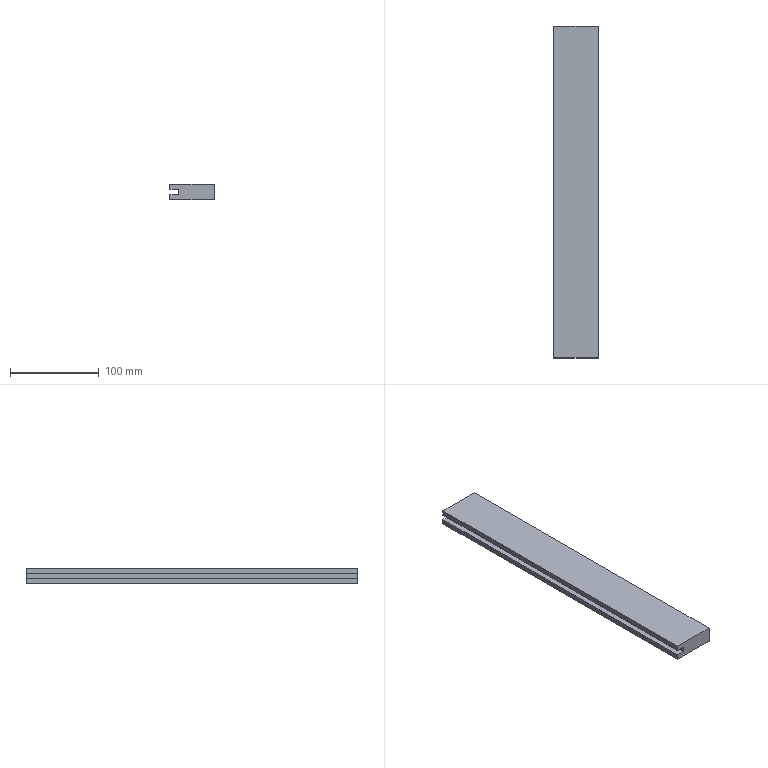Part | STEP file | Superstructure_1 | 1 solid | 10 faces | box 50 x 374 x 18 mm | volume 314160 mm3 | plane 10
STEP:
#1=CARTESIAN_POINT('',(0.,0.,0.));
#2=DIRECTION('',(0.,0.,1.));
#3=DIRECTION('',(1.,0.,0.));
#4=AXIS2_PLACEMENT_3D('',#1,#2,#3);
#5=CARTESIAN_POINT('',(-25.,187.,-3.));
#6=VERTEX_POINT('',#5);
#7=CARTESIAN_POINT('',(-25.,-187.,-3.));
#8=VERTEX_POINT('',#7);
#9=CARTESIAN_POINT('',(-25.,187.,-3.));
#10=DIRECTION('',(0.,-1.,0.));
#11=VECTOR('',#10,1.);
#12=LINE('',#9,#11);
#13=CARTESIAN_POINT('',(-25.,187.,-3.));
#14=DIRECTION('',(1.,0.,0.));
#15=DIRECTION('',(0.,0.,-1.));
#16=AXIS2_PLACEMENT_3D('',#13,#14,#15);
#17=PLANE('',#16);
#18=CARTESIAN_POINT('',(0.,0.));
#19=DIRECTION('',(0.,-1.));
#20=VECTOR('',#19,1.);
#21=LINE('',#18,#20);
#22=(GEOMETRIC_REPRESENTATION_CONTEXT(2)PARAMETRIC_REPRESENTATION_CONTEXT()REPRESENTATION_CONTEXT('',''));
#23=DEFINITIONAL_REPRESENTATION('',(#21),#22);
#24=PCURVE('',#17,#23);
#25=CARTESIAN_POINT('',(-25.,187.,-3.));
#26=DIRECTION('',(0.,0.,1.));
#27=DIRECTION('',(1.,0.,0.));
#28=AXIS2_PLACEMENT_3D('',#25,#26,#27);
#29=PLANE('',#28);
#30=CARTESIAN_POINT('',(0.,0.));
#31=DIRECTION('',(0.,-1.));
#32=VECTOR('',#31,1.);
#33=LINE('',#30,#32);
#34=(GEOMETRIC_REPRESENTATION_CONTEXT(2)PARAMETRIC_REPRESENTATION_CONTEXT()REPRESENTATION_CONTEXT('',''));
#35=DEFINITIONAL_REPRESENTATION('',(#33),#34);
#36=PCURVE('',#29,#35);
#37=SURFACE_CURVE('',#12,(#24,#36),.PCURVE_S1.);
#38=EDGE_CURVE('',#6,#8,#37,.T.);
#39=ORIENTED_EDGE('',*,*,#38,.T.);
#40=CARTESIAN_POINT('',(-25.,-187.,-9.));
#41=VERTEX_POINT('',#40);
#42=CARTESIAN_POINT('',(-25.,-187.,-3.));
#43=DIRECTION('',(0.,0.,-1.));
#44=VECTOR('',#43,1.);
#45=LINE('',#42,#44);
#46=CARTESIAN_POINT('',(0.,-374.));
#47=DIRECTION('',(1.,0.));
#48=VECTOR('',#47,1.);
#49=LINE('',#46,#48);
#50=(GEOMETRIC_REPRESENTATION_CONTEXT(2)PARAMETRIC_REPRESENTATION_CONTEXT()REPRESENTATION_CONTEXT('',''));
#51=DEFINITIONAL_REPRESENTATION('',(#49),#50);
#52=PCURVE('',#17,#51);
#53=CARTESIAN_POINT('',(-2.179,-187.,0.));
#54=DIRECTION('',(0.,1.,0.));
#55=DIRECTION('',(0.,0.,1.));
#56=AXIS2_PLACEMENT_3D('',#53,#54,#55);
#57=PLANE('',#56);
#58=CARTESIAN_POINT('',(-3.,-22.821));
#59=DIRECTION('',(-1.,0.));
#60=VECTOR('',#59,1.);
#61=LINE('',#58,#60);
#62=(GEOMETRIC_REPRESENTATION_CONTEXT(2)PARAMETRIC_REPRESENTATION_CONTEXT()REPRESENTATION_CONTEXT('',''));
#63=DEFINITIONAL_REPRESENTATION('',(#61),#62);
#64=PCURVE('',#57,#63);
#65=SURFACE_CURVE('',#45,(#52,#64),.PCURVE_S1.);
#66=EDGE_CURVE('',#8,#41,#65,.T.);
#67=ORIENTED_EDGE('',*,*,#66,.T.);
#68=CARTESIAN_POINT('',(-25.,187.,-9.));
#69=VERTEX_POINT('',#68);
#70=CARTESIAN_POINT('',(-25.,187.,-9.));
#71=DIRECTION('',(0.,-1.,0.));
#72=VECTOR('',#71,1.);
#73=LINE('',#70,#72);
#74=CARTESIAN_POINT('',(6.,0.));
#75=DIRECTION('',(0.,-1.));
#76=VECTOR('',#75,1.);
#77=LINE('',#74,#76);
#78=(GEOMETRIC_REPRESENTATION_CONTEXT(2)PARAMETRIC_REPRESENTATION_CONTEXT()REPRESENTATION_CONTEXT('',''));
#79=DEFINITIONAL_REPRESENTATION('',(#77),#78);
#80=PCURVE('',#17,#79);
#81=CARTESIAN_POINT('',(-25.,187.,-9.));
#82=DIRECTION('',(0.,0.,1.));
#83=DIRECTION('',(1.,0.,0.));
#84=AXIS2_PLACEMENT_3D('',#81,#82,#83);
#85=PLANE('',#84);
#86=CARTESIAN_POINT('',(0.,0.));
#87=DIRECTION('',(0.,-1.));
#88=VECTOR('',#87,1.);
#89=LINE('',#86,#88);
#90=(GEOMETRIC_REPRESENTATION_CONTEXT(2)PARAMETRIC_REPRESENTATION_CONTEXT()REPRESENTATION_CONTEXT('',''));
#91=DEFINITIONAL_REPRESENTATION('',(#89),#90);
#92=PCURVE('',#85,#91);
#93=SURFACE_CURVE('',#73,(#80,#92),.PCURVE_S1.);
#94=EDGE_CURVE('',#69,#41,#93,.T.);
#95=ORIENTED_EDGE('',*,*,#94,.F.);
#96=CARTESIAN_POINT('',(-25.,187.,-3.));
#97=DIRECTION('',(0.,0.,-1.));
#98=VECTOR('',#97,1.);
#99=LINE('',#96,#98);
#100=CARTESIAN_POINT('',(0.,0.));
#101=DIRECTION('',(1.,0.));
#102=VECTOR('',#101,1.);
#103=LINE('',#100,#102);
#104=(GEOMETRIC_REPRESENTATION_CONTEXT(2)PARAMETRIC_REPRESENTATION_CONTEXT()REPRESENTATION_CONTEXT('',''));
#105=DEFINITIONAL_REPRESENTATION('',(#103),#104);
#106=PCURVE('',#17,#105);
#107=CARTESIAN_POINT('',(-2.179,187.,0.));
#108=DIRECTION('',(0.,1.,0.));
#109=DIRECTION('',(0.,0.,1.));
#110=AXIS2_PLACEMENT_3D('',#107,#108,#109);
#111=PLANE('',#110);
#112=CARTESIAN_POINT('',(-3.,-22.821));
#113=DIRECTION('',(-1.,0.));
#114=VECTOR('',#113,1.);
#115=LINE('',#112,#114);
#116=(GEOMETRIC_REPRESENTATION_CONTEXT(2)PARAMETRIC_REPRESENTATION_CONTEXT()REPRESENTATION_CONTEXT('',''));
#117=DEFINITIONAL_REPRESENTATION('',(#115),#116);
#118=PCURVE('',#111,#117);
#119=SURFACE_CURVE('',#99,(#106,#118),.PCURVE_S1.);
#120=EDGE_CURVE('',#6,#69,#119,.T.);
#121=ORIENTED_EDGE('',*,*,#120,.F.);
#122=EDGE_LOOP('',(#39,#67,#95,#121));
#123=FACE_BOUND('',#122,.F.);
#124=ADVANCED_FACE('',(#123),#17,.F.);
#125=ORIENTED_EDGE('',*,*,#94,.T.);
#126=CARTESIAN_POINT('',(25.,-187.,-9.));
#127=VERTEX_POINT('',#126);
#128=CARTESIAN_POINT('',(-25.,-187.,-9.));
#129=DIRECTION('',(1.,0.,0.));
#130=VECTOR('',#129,1.);
#131=LINE('',#128,#130);
#132=CARTESIAN_POINT('',(0.,-374.));
#133=DIRECTION('',(1.,0.));
#134=VECTOR('',#133,1.);
#135=LINE('',#132,#134);
#136=(GEOMETRIC_REPRESENTATION_CONTEXT(2)PARAMETRIC_REPRESENTATION_CONTEXT()REPRESENTATION_CONTEXT('',''));
#137=DEFINITIONAL_REPRESENTATION('',(#135),#136);
#138=PCURVE('',#85,#137);
#139=CARTESIAN_POINT('',(-9.,-22.821));
#140=DIRECTION('',(0.,1.));
#141=VECTOR('',#140,1.);
#142=LINE('',#139,#141);
#143=(GEOMETRIC_REPRESENTATION_CONTEXT(2)PARAMETRIC_REPRESENTATION_CONTEXT()REPRESENTATION_CONTEXT('',''));
#144=DEFINITIONAL_REPRESENTATION('',(#142),#143);
#145=PCURVE('',#57,#144);
#146=SURFACE_CURVE('',#131,(#138,#145),.PCURVE_S1.);
#147=EDGE_CURVE('',#41,#127,#146,.T.);
#148=ORIENTED_EDGE('',*,*,#147,.T.);
#149=CARTESIAN_POINT('',(25.,187.,-9.));
#150=VERTEX_POINT('',#149);
#151=CARTESIAN_POINT('',(25.,187.,-9.));
#152=DIRECTION('',(0.,-1.,0.));
#153=VECTOR('',#152,1.);
#154=LINE('',#151,#153);
#155=CARTESIAN_POINT('',(50.,0.));
#156=DIRECTION('',(0.,-1.));
#157=VECTOR('',#156,1.);
#158=LINE('',#155,#157);
#159=(GEOMETRIC_REPRESENTATION_CONTEXT(2)PARAMETRIC_REPRESENTATION_CONTEXT()REPRESENTATION_CONTEXT('',''));
#160=DEFINITIONAL_REPRESENTATION('',(#158),#159);
#161=PCURVE('',#85,#160);
#162=CARTESIAN_POINT('',(25.,187.,-9.));
#163=DIRECTION('',(-1.,0.,0.));
#164=DIRECTION('',(0.,0.,1.));
#165=AXIS2_PLACEMENT_3D('',#162,#163,#164);
#166=PLANE('',#165);
#167=CARTESIAN_POINT('',(0.,0.));
#168=DIRECTION('',(0.,-1.));
#169=VECTOR('',#168,1.);
#170=LINE('',#167,#169);
#171=(GEOMETRIC_REPRESENTATION_CONTEXT(2)PARAMETRIC_REPRESENTATION_CONTEXT()REPRESENTATION_CONTEXT('',''));
#172=DEFINITIONAL_REPRESENTATION('',(#170),#171);
#173=PCURVE('',#166,#172);
#174=SURFACE_CURVE('',#154,(#161,#173),.PCURVE_S1.);
#175=EDGE_CURVE('',#150,#127,#174,.T.);
#176=ORIENTED_EDGE('',*,*,#175,.F.);
#177=CARTESIAN_POINT('',(-25.,187.,-9.));
#178=DIRECTION('',(1.,0.,0.));
#179=VECTOR('',#178,1.);
#180=LINE('',#177,#179);
#181=CARTESIAN_POINT('',(0.,0.));
#182=DIRECTION('',(1.,0.));
#183=VECTOR('',#182,1.);
#184=LINE('',#181,#183);
#185=(GEOMETRIC_REPRESENTATION_CONTEXT(2)PARAMETRIC_REPRESENTATION_CONTEXT()REPRESENTATION_CONTEXT('',''));
#186=DEFINITIONAL_REPRESENTATION('',(#184),#185);
#187=PCURVE('',#85,#186);
#188=CARTESIAN_POINT('',(-9.,-22.821));
#189=DIRECTION('',(0.,1.));
#190=VECTOR('',#189,1.);
#191=LINE('',#188,#190);
#192=(GEOMETRIC_REPRESENTATION_CONTEXT(2)PARAMETRIC_REPRESENTATION_CONTEXT()REPRESENTATION_CONTEXT('',''));
#193=DEFINITIONAL_REPRESENTATION('',(#191),#192);
#194=PCURVE('',#111,#193);
#195=SURFACE_CURVE('',#180,(#187,#194),.PCURVE_S1.);
#196=EDGE_CURVE('',#69,#150,#195,.T.);
#197=ORIENTED_EDGE('',*,*,#196,.F.);
#198=EDGE_LOOP('',(#125,#148,#176,#197));
#199=FACE_BOUND('',#198,.F.);
#200=ADVANCED_FACE('',(#199),#85,.F.);
#201=ORIENTED_EDGE('',*,*,#175,.T.);
#202=CARTESIAN_POINT('',(25.,-187.,9.));
#203=VERTEX_POINT('',#202);
#204=CARTESIAN_POINT('',(25.,-187.,-9.));
#205=DIRECTION('',(0.,0.,1.));
#206=VECTOR('',#205,1.);
#207=LINE('',#204,#206);
#208=CARTESIAN_POINT('',(0.,-374.));
#209=DIRECTION('',(1.,0.));
#210=VECTOR('',#209,1.);
#211=LINE('',#208,#210);
#212=(GEOMETRIC_REPRESENTATION_CONTEXT(2)PARAMETRIC_REPRESENTATION_CONTEXT()REPRESENTATION_CONTEXT('',''));
#213=DEFINITIONAL_REPRESENTATION('',(#211),#212);
#214=PCURVE('',#166,#213);
#215=CARTESIAN_POINT('',(-9.,27.179));
#216=DIRECTION('',(1.,0.));
#217=VECTOR('',#216,1.);
#218=LINE('',#215,#217);
#219=(GEOMETRIC_REPRESENTATION_CONTEXT(2)PARAMETRIC_REPRESENTATION_CONTEXT()REPRESENTATION_CONTEXT('',''));
#220=DEFINITIONAL_REPRESENTATION('',(#218),#219);
#221=PCURVE('',#57,#220);
#222=SURFACE_CURVE('',#207,(#214,#221),.PCURVE_S1.);
#223=EDGE_CURVE('',#127,#203,#222,.T.);
#224=ORIENTED_EDGE('',*,*,#223,.T.);
#225=CARTESIAN_POINT('',(25.,187.,9.));
#226=VERTEX_POINT('',#225);
#227=CARTESIAN_POINT('',(25.,187.,9.));
#228=DIRECTION('',(0.,-1.,0.));
#229=VECTOR('',#228,1.);
#230=LINE('',#227,#229);
#231=CARTESIAN_POINT('',(18.,0.));
#232=DIRECTION('',(0.,-1.));
#233=VECTOR('',#232,1.);
#234=LINE('',#231,#233);
#235=(GEOMETRIC_REPRESENTATION_CONTEXT(2)PARAMETRIC_REPRESENTATION_CONTEXT()REPRESENTATION_CONTEXT('',''));
#236=DEFINITIONAL_REPRESENTATION('',(#234),#235);
#237=PCURVE('',#166,#236);
#238=CARTESIAN_POINT('',(25.,187.,9.));
#239=DIRECTION('',(0.,0.,-1.));
#240=DIRECTION('',(-1.,0.,0.));
#241=AXIS2_PLACEMENT_3D('',#238,#239,#240);
#242=PLANE('',#241);
#243=CARTESIAN_POINT('',(0.,0.));
#244=DIRECTION('',(0.,-1.));
#245=VECTOR('',#244,1.);
#246=LINE('',#243,#245);
#247=(GEOMETRIC_REPRESENTATION_CONTEXT(2)PARAMETRIC_REPRESENTATION_CONTEXT()REPRESENTATION_CONTEXT('',''));
#248=DEFINITIONAL_REPRESENTATION('',(#246),#247);
#249=PCURVE('',#242,#248);
#250=SURFACE_CURVE('',#230,(#237,#249),.PCURVE_S1.);
#251=EDGE_CURVE('',#226,#203,#250,.T.);
#252=ORIENTED_EDGE('',*,*,#251,.F.);
#253=CARTESIAN_POINT('',(25.,187.,-9.));
#254=DIRECTION('',(0.,0.,1.));
#255=VECTOR('',#254,1.);
#256=LINE('',#253,#255);
#257=CARTESIAN_POINT('',(0.,0.));
#258=DIRECTION('',(1.,0.));
#259=VECTOR('',#258,1.);
#260=LINE('',#257,#259);
#261=(GEOMETRIC_REPRESENTATION_CONTEXT(2)PARAMETRIC_REPRESENTATION_CONTEXT()REPRESENTATION_CONTEXT('',''));
#262=DEFINITIONAL_REPRESENTATION('',(#260),#261);
#263=PCURVE('',#166,#262);
#264=CARTESIAN_POINT('',(-9.,27.179));
#265=DIRECTION('',(1.,0.));
#266=VECTOR('',#265,1.);
#267=LINE('',#264,#266);
#268=(GEOMETRIC_REPRESENTATION_CONTEXT(2)PARAMETRIC_REPRESENTATION_CONTEXT()REPRESENTATION_CONTEXT('',''));
#269=DEFINITIONAL_REPRESENTATION('',(#267),#268);
#270=PCURVE('',#111,#269);
#271=SURFACE_CURVE('',#256,(#263,#270),.PCURVE_S1.);
#272=EDGE_CURVE('',#150,#226,#271,.T.);
#273=ORIENTED_EDGE('',*,*,#272,.F.);
#274=EDGE_LOOP('',(#201,#224,#252,#273));
#275=FACE_BOUND('',#274,.F.);
#276=ADVANCED_FACE('',(#275),#166,.F.);
#277=ORIENTED_EDGE('',*,*,#251,.T.);
#278=CARTESIAN_POINT('',(-25.,-187.,9.));
#279=VERTEX_POINT('',#278);
#280=CARTESIAN_POINT('',(25.,-187.,9.));
#281=DIRECTION('',(-1.,0.,0.));
#282=VECTOR('',#281,1.);
#283=LINE('',#280,#282);
#284=CARTESIAN_POINT('',(0.,-374.));
#285=DIRECTION('',(1.,0.));
#286=VECTOR('',#285,1.);
#287=LINE('',#284,#286);
#288=(GEOMETRIC_REPRESENTATION_CONTEXT(2)PARAMETRIC_REPRESENTATION_CONTEXT()REPRESENTATION_CONTEXT('',''));
#289=DEFINITIONAL_REPRESENTATION('',(#287),#288);
#290=PCURVE('',#242,#289);
#291=CARTESIAN_POINT('',(9.,27.179));
#292=DIRECTION('',(0.,-1.));
#293=VECTOR('',#292,1.);
#294=LINE('',#291,#293);
#295=(GEOMETRIC_REPRESENTATION_CONTEXT(2)PARAMETRIC_REPRESENTATION_CONTEXT()REPRESENTATION_CONTEXT('',''));
#296=DEFINITIONAL_REPRESENTATION('',(#294),#295);
#297=PCURVE('',#57,#296);
#298=SURFACE_CURVE('',#283,(#290,#297),.PCURVE_S1.);
#299=EDGE_CURVE('',#203,#279,#298,.T.);
#300=ORIENTED_EDGE('',*,*,#299,.T.);
#301=CARTESIAN_POINT('',(-25.,187.,9.));
#302=VERTEX_POINT('',#301);
#303=CARTESIAN_POINT('',(-25.,187.,9.));
#304=DIRECTION('',(0.,-1.,0.));
#305=VECTOR('',#304,1.);
#306=LINE('',#303,#305);
#307=CARTESIAN_POINT('',(50.,0.));
#308=DIRECTION('',(0.,-1.));
#309=VECTOR('',#308,1.);
#310=LINE('',#307,#309);
#311=(GEOMETRIC_REPRESENTATION_CONTEXT(2)PARAMETRIC_REPRESENTATION_CONTEXT()REPRESENTATION_CONTEXT('',''));
#312=DEFINITIONAL_REPRESENTATION('',(#310),#311);
#313=PCURVE('',#242,#312);
#314=CARTESIAN_POINT('',(-25.,187.,9.));
#315=DIRECTION('',(1.,0.,0.));
#316=DIRECTION('',(0.,0.,-1.));
#317=AXIS2_PLACEMENT_3D('',#314,#315,#316);
#318=PLANE('',#317);
#319=CARTESIAN_POINT('',(0.,0.));
#320=DIRECTION('',(0.,-1.));
#321=VECTOR('',#320,1.);
#322=LINE('',#319,#321);
#323=(GEOMETRIC_REPRESENTATION_CONTEXT(2)PARAMETRIC_REPRESENTATION_CONTEXT()REPRESENTATION_CONTEXT('',''));
#324=DEFINITIONAL_REPRESENTATION('',(#322),#323);
#325=PCURVE('',#318,#324);
#326=SURFACE_CURVE('',#306,(#313,#325),.PCURVE_S1.);
#327=EDGE_CURVE('',#302,#279,#326,.T.);
#328=ORIENTED_EDGE('',*,*,#327,.F.);
#329=CARTESIAN_POINT('',(25.,187.,9.));
#330=DIRECTION('',(-1.,0.,0.));
#331=VECTOR('',#330,1.);
#332=LINE('',#329,#331);
#333=CARTESIAN_POINT('',(0.,0.));
#334=DIRECTION('',(1.,0.));
#335=VECTOR('',#334,1.);
#336=LINE('',#333,#335);
#337=(GEOMETRIC_REPRESENTATION_CONTEXT(2)PARAMETRIC_REPRESENTATION_CONTEXT()REPRESENTATION_CONTEXT('',''));
#338=DEFINITIONAL_REPRESENTATION('',(#336),#337);
#339=PCURVE('',#242,#338);
#340=CARTESIAN_POINT('',(9.,27.179));
#341=DIRECTION('',(0.,-1.));
#342=VECTOR('',#341,1.);
#343=LINE('',#340,#342);
#344=(GEOMETRIC_REPRESENTATION_CONTEXT(2)PARAMETRIC_REPRESENTATION_CONTEXT()REPRESENTATION_CONTEXT('',''));
#345=DEFINITIONAL_REPRESENTATION('',(#343),#344);
#346=PCURVE('',#111,#345);
#347=SURFACE_CURVE('',#332,(#339,#346),.PCURVE_S1.);
#348=EDGE_CURVE('',#226,#302,#347,.T.);
#349=ORIENTED_EDGE('',*,*,#348,.F.);
#350=EDGE_LOOP('',(#277,#300,#328,#349));
#351=FACE_BOUND('',#350,.F.);
#352=ADVANCED_FACE('',(#351),#242,.F.);
#353=ORIENTED_EDGE('',*,*,#327,.T.);
#354=CARTESIAN_POINT('',(-25.,-187.,3.));
#355=VERTEX_POINT('',#354);
#356=CARTESIAN_POINT('',(-25.,-187.,9.));
#357=DIRECTION('',(0.,0.,-1.));
#358=VECTOR('',#357,1.);
#359=LINE('',#356,#358);
#360=CARTESIAN_POINT('',(0.,-374.));
#361=DIRECTION('',(1.,0.));
#362=VECTOR('',#361,1.);
#363=LINE('',#360,#362);
#364=(GEOMETRIC_REPRESENTATION_CONTEXT(2)PARAMETRIC_REPRESENTATION_CONTEXT()REPRESENTATION_CONTEXT('',''));
#365=DEFINITIONAL_REPRESENTATION('',(#363),#364);
#366=PCURVE('',#318,#365);
#367=CARTESIAN_POINT('',(9.,-22.821));
#368=DIRECTION('',(-1.,0.));
#369=VECTOR('',#368,1.);
#370=LINE('',#367,#369);
#371=(GEOMETRIC_REPRESENTATION_CONTEXT(2)PARAMETRIC_REPRESENTATION_CONTEXT()REPRESENTATION_CONTEXT('',''));
#372=DEFINITIONAL_REPRESENTATION('',(#370),#371);
#373=PCURVE('',#57,#372);
#374=SURFACE_CURVE('',#359,(#366,#373),.PCURVE_S1.);
#375=EDGE_CURVE('',#279,#355,#374,.T.);
#376=ORIENTED_EDGE('',*,*,#375,.T.);
#377=CARTESIAN_POINT('',(-25.,187.,3.));
#378=VERTEX_POINT('',#377);
#379=CARTESIAN_POINT('',(-25.,187.,3.));
#380=DIRECTION('',(0.,-1.,0.));
#381=VECTOR('',#380,1.);
#382=LINE('',#379,#381);
#383=CARTESIAN_POINT('',(6.,0.));
#384=DIRECTION('',(0.,-1.));
#385=VECTOR('',#384,1.);
#386=LINE('',#383,#385);
#387=(GEOMETRIC_REPRESENTATION_CONTEXT(2)PARAMETRIC_REPRESENTATION_CONTEXT()REPRESENTATION_CONTEXT('',''));
#388=DEFINITIONAL_REPRESENTATION('',(#386),#387);
#389=PCURVE('',#318,#388);
#390=CARTESIAN_POINT('',(-15.,187.,3.));
#391=DIRECTION('',(0.,0.,-1.));
#392=DIRECTION('',(-1.,0.,0.));
#393=AXIS2_PLACEMENT_3D('',#390,#391,#392);
#394=PLANE('',#393);
#395=CARTESIAN_POINT('',(10.,0.));
#396=DIRECTION('',(0.,-1.));
#397=VECTOR('',#396,1.);
#398=LINE('',#395,#397);
#399=(GEOMETRIC_REPRESENTATION_CONTEXT(2)PARAMETRIC_REPRESENTATION_CONTEXT()REPRESENTATION_CONTEXT('',''));
#400=DEFINITIONAL_REPRESENTATION('',(#398),#399);
#401=PCURVE('',#394,#400);
#402=SURFACE_CURVE('',#382,(#389,#401),.PCURVE_S1.);
#403=EDGE_CURVE('',#378,#355,#402,.T.);
#404=ORIENTED_EDGE('',*,*,#403,.F.);
#405=CARTESIAN_POINT('',(-25.,187.,9.));
#406=DIRECTION('',(0.,0.,-1.));
#407=VECTOR('',#406,1.);
#408=LINE('',#405,#407);
#409=CARTESIAN_POINT('',(0.,0.));
#410=DIRECTION('',(1.,0.));
#411=VECTOR('',#410,1.);
#412=LINE('',#409,#411);
#413=(GEOMETRIC_REPRESENTATION_CONTEXT(2)PARAMETRIC_REPRESENTATION_CONTEXT()REPRESENTATION_CONTEXT('',''));
#414=DEFINITIONAL_REPRESENTATION('',(#412),#413);
#415=PCURVE('',#318,#414);
#416=CARTESIAN_POINT('',(9.,-22.821));
#417=DIRECTION('',(-1.,0.));
#418=VECTOR('',#417,1.);
#419=LINE('',#416,#418);
#420=(GEOMETRIC_REPRESENTATION_CONTEXT(2)PARAMETRIC_REPRESENTATION_CONTEXT()REPRESENTATION_CONTEXT('',''));
#421=DEFINITIONAL_REPRESENTATION('',(#419),#420);
#422=PCURVE('',#111,#421);
#423=SURFACE_CURVE('',#408,(#415,#422),.PCURVE_S1.);
#424=EDGE_CURVE('',#302,#378,#423,.T.);
#425=ORIENTED_EDGE('',*,*,#424,.F.);
#426=EDGE_LOOP('',(#353,#376,#404,#425));
#427=FACE_BOUND('',#426,.F.);
#428=ADVANCED_FACE('',(#427),#318,.F.);
#429=CARTESIAN_POINT('',(-15.,187.,3.));
#430=VERTEX_POINT('',#429);
#431=CARTESIAN_POINT('',(-15.,-187.,3.));
#432=VERTEX_POINT('',#431);
#433=CARTESIAN_POINT('',(-15.,187.,3.));
#434=DIRECTION('',(0.,-1.,0.));
#435=VECTOR('',#434,1.);
#436=LINE('',#433,#435);
#437=CARTESIAN_POINT('',(0.,0.));
#438=DIRECTION('',(0.,-1.));
#439=VECTOR('',#438,1.);
#440=LINE('',#437,#439);
#441=(GEOMETRIC_REPRESENTATION_CONTEXT(2)PARAMETRIC_REPRESENTATION_CONTEXT()REPRESENTATION_CONTEXT('',''));
#442=DEFINITIONAL_REPRESENTATION('',(#440),#441);
#443=PCURVE('',#394,#442);
#444=CARTESIAN_POINT('',(-15.,187.,-3.));
#445=DIRECTION('',(-1.,0.,0.));
#446=DIRECTION('',(0.,0.,1.));
#447=AXIS2_PLACEMENT_3D('',#444,#445,#446);
#448=PLANE('',#447);
#449=CARTESIAN_POINT('',(6.,0.));
#450=DIRECTION('',(0.,-1.));
#451=VECTOR('',#450,1.);
#452=LINE('',#449,#451);
#453=(GEOMETRIC_REPRESENTATION_CONTEXT(2)PARAMETRIC_REPRESENTATION_CONTEXT()REPRESENTATION_CONTEXT('',''));
#454=DEFINITIONAL_REPRESENTATION('',(#452),#453);
#455=PCURVE('',#448,#454);
#456=SURFACE_CURVE('',#436,(#443,#455),.PCURVE_S1.);
#457=EDGE_CURVE('',#430,#432,#456,.T.);
#458=ORIENTED_EDGE('',*,*,#457,.T.);
#459=CARTESIAN_POINT('',(-15.,-187.,3.));
#460=DIRECTION('',(-1.,0.,0.));
#461=VECTOR('',#460,1.);
#462=LINE('',#459,#461);
#463=CARTESIAN_POINT('',(0.,-374.));
#464=DIRECTION('',(1.,0.));
#465=VECTOR('',#464,1.);
#466=LINE('',#463,#465);
#467=(GEOMETRIC_REPRESENTATION_CONTEXT(2)PARAMETRIC_REPRESENTATION_CONTEXT()REPRESENTATION_CONTEXT('',''));
#468=DEFINITIONAL_REPRESENTATION('',(#466),#467);
#469=PCURVE('',#394,#468);
#470=CARTESIAN_POINT('',(3.,-12.821));
#471=DIRECTION('',(0.,-1.));
#472=VECTOR('',#471,1.);
#473=LINE('',#470,#472);
#474=(GEOMETRIC_REPRESENTATION_CONTEXT(2)PARAMETRIC_REPRESENTATION_CONTEXT()REPRESENTATION_CONTEXT('',''));
#475=DEFINITIONAL_REPRESENTATION('',(#473),#474);
#476=PCURVE('',#57,#475);
#477=SURFACE_CURVE('',#462,(#469,#476),.PCURVE_S1.);
#478=EDGE_CURVE('',#432,#355,#477,.T.);
#479=ORIENTED_EDGE('',*,*,#478,.T.);
#480=ORIENTED_EDGE('',*,*,#403,.F.);
#481=CARTESIAN_POINT('',(-15.,187.,3.));
#482=DIRECTION('',(-1.,0.,0.));
#483=VECTOR('',#482,1.);
#484=LINE('',#481,#483);
#485=CARTESIAN_POINT('',(0.,0.));
#486=DIRECTION('',(1.,0.));
#487=VECTOR('',#486,1.);
#488=LINE('',#485,#487);
#489=(GEOMETRIC_REPRESENTATION_CONTEXT(2)PARAMETRIC_REPRESENTATION_CONTEXT()REPRESENTATION_CONTEXT('',''));
#490=DEFINITIONAL_REPRESENTATION('',(#488),#489);
#491=PCURVE('',#394,#490);
#492=CARTESIAN_POINT('',(3.,-12.821));
#493=DIRECTION('',(0.,-1.));
#494=VECTOR('',#493,1.);
#495=LINE('',#492,#494);
#496=(GEOMETRIC_REPRESENTATION_CONTEXT(2)PARAMETRIC_REPRESENTATION_CONTEXT()REPRESENTATION_CONTEXT('',''));
#497=DEFINITIONAL_REPRESENTATION('',(#495),#496);
#498=PCURVE('',#111,#497);
#499=SURFACE_CURVE('',#484,(#491,#498),.PCURVE_S1.);
#500=EDGE_CURVE('',#430,#378,#499,.T.);
#501=ORIENTED_EDGE('',*,*,#500,.F.);
#502=EDGE_LOOP('',(#458,#479,#480,#501));
#503=FACE_BOUND('',#502,.T.);
#504=ADVANCED_FACE('',(#503),#394,.T.);
#505=CARTESIAN_POINT('',(-15.,187.,-3.));
#506=VERTEX_POINT('',#505);
#507=CARTESIAN_POINT('',(-15.,-187.,-3.));
#508=VERTEX_POINT('',#507);
#509=CARTESIAN_POINT('',(-15.,187.,-3.));
#510=DIRECTION('',(0.,-1.,0.));
#511=VECTOR('',#510,1.);
#512=LINE('',#509,#511);
#513=CARTESIAN_POINT('',(0.,0.));
#514=DIRECTION('',(0.,-1.));
#515=VECTOR('',#514,1.);
#516=LINE('',#513,#515);
#517=(GEOMETRIC_REPRESENTATION_CONTEXT(2)PARAMETRIC_REPRESENTATION_CONTEXT()REPRESENTATION_CONTEXT('',''));
#518=DEFINITIONAL_REPRESENTATION('',(#516),#517);
#519=PCURVE('',#448,#518);
#520=CARTESIAN_POINT('',(10.,0.));
#521=DIRECTION('',(0.,-1.));
#522=VECTOR('',#521,1.);
#523=LINE('',#520,#522);
#524=(GEOMETRIC_REPRESENTATION_CONTEXT(2)PARAMETRIC_REPRESENTATION_CONTEXT()REPRESENTATION_CONTEXT('',''));
#525=DEFINITIONAL_REPRESENTATION('',(#523),#524);
#526=PCURVE('',#29,#525);
#527=SURFACE_CURVE('',#512,(#519,#526),.PCURVE_S1.);
#528=EDGE_CURVE('',#506,#508,#527,.T.);
#529=ORIENTED_EDGE('',*,*,#528,.T.);
#530=CARTESIAN_POINT('',(-15.,-187.,-3.));
#531=DIRECTION('',(0.,0.,1.));
#532=VECTOR('',#531,1.);
#533=LINE('',#530,#532);
#534=CARTESIAN_POINT('',(0.,-374.));
#535=DIRECTION('',(1.,0.));
#536=VECTOR('',#535,1.);
#537=LINE('',#534,#536);
#538=(GEOMETRIC_REPRESENTATION_CONTEXT(2)PARAMETRIC_REPRESENTATION_CONTEXT()REPRESENTATION_CONTEXT('',''));
#539=DEFINITIONAL_REPRESENTATION('',(#537),#538);
#540=PCURVE('',#448,#539);
#541=CARTESIAN_POINT('',(-3.,-12.821));
#542=DIRECTION('',(1.,0.));
#543=VECTOR('',#542,1.);
#544=LINE('',#541,#543);
#545=(GEOMETRIC_REPRESENTATION_CONTEXT(2)PARAMETRIC_REPRESENTATION_CONTEXT()REPRESENTATION_CONTEXT('',''));
#546=DEFINITIONAL_REPRESENTATION('',(#544),#545);
#547=PCURVE('',#57,#546);
#548=SURFACE_CURVE('',#533,(#540,#547),.PCURVE_S1.);
#549=EDGE_CURVE('',#508,#432,#548,.T.);
#550=ORIENTED_EDGE('',*,*,#549,.T.);
#551=ORIENTED_EDGE('',*,*,#457,.F.);
#552=CARTESIAN_POINT('',(-15.,187.,-3.));
#553=DIRECTION('',(0.,0.,1.));
#554=VECTOR('',#553,1.);
#555=LINE('',#552,#554);
#556=CARTESIAN_POINT('',(0.,0.));
#557=DIRECTION('',(1.,0.));
#558=VECTOR('',#557,1.);
#559=LINE('',#556,#558);
#560=(GEOMETRIC_REPRESENTATION_CONTEXT(2)PARAMETRIC_REPRESENTATION_CONTEXT()REPRESENTATION_CONTEXT('',''));
#561=DEFINITIONAL_REPRESENTATION('',(#559),#560);
#562=PCURVE('',#448,#561);
#563=CARTESIAN_POINT('',(-3.,-12.821));
#564=DIRECTION('',(1.,0.));
#565=VECTOR('',#564,1.);
#566=LINE('',#563,#565);
#567=(GEOMETRIC_REPRESENTATION_CONTEXT(2)PARAMETRIC_REPRESENTATION_CONTEXT()REPRESENTATION_CONTEXT('',''));
#568=DEFINITIONAL_REPRESENTATION('',(#566),#567);
#569=PCURVE('',#111,#568);
#570=SURFACE_CURVE('',#555,(#562,#569),.PCURVE_S1.);
#571=EDGE_CURVE('',#506,#430,#570,.T.);
#572=ORIENTED_EDGE('',*,*,#571,.F.);
#573=EDGE_LOOP('',(#529,#550,#551,#572));
#574=FACE_BOUND('',#573,.T.);
#575=ADVANCED_FACE('',(#574),#448,.T.);
#576=ORIENTED_EDGE('',*,*,#38,.T.);
#577=CARTESIAN_POINT('',(-25.,-187.,-3.));
#578=DIRECTION('',(1.,0.,0.));
#579=VECTOR('',#578,1.);
#580=LINE('',#577,#579);
#581=CARTESIAN_POINT('',(0.,-374.));
#582=DIRECTION('',(1.,0.));
#583=VECTOR('',#582,1.);
#584=LINE('',#581,#583);
#585=(GEOMETRIC_REPRESENTATION_CONTEXT(2)PARAMETRIC_REPRESENTATION_CONTEXT()REPRESENTATION_CONTEXT('',''));
#586=DEFINITIONAL_REPRESENTATION('',(#584),#585);
#587=PCURVE('',#29,#586);
#588=CARTESIAN_POINT('',(-3.,-22.821));
#589=DIRECTION('',(0.,1.));
#590=VECTOR('',#589,1.);
#591=LINE('',#588,#590);
#592=(GEOMETRIC_REPRESENTATION_CONTEXT(2)PARAMETRIC_REPRESENTATION_CONTEXT()REPRESENTATION_CONTEXT('',''));
#593=DEFINITIONAL_REPRESENTATION('',(#591),#592);
#594=PCURVE('',#57,#593);
#595=SURFACE_CURVE('',#580,(#587,#594),.PCURVE_S1.);
#596=EDGE_CURVE('',#8,#508,#595,.T.);
#597=ORIENTED_EDGE('',*,*,#596,.T.);
#598=ORIENTED_EDGE('',*,*,#528,.F.);
#599=CARTESIAN_POINT('',(-25.,187.,-3.));
#600=DIRECTION('',(1.,0.,0.));
#601=VECTOR('',#600,1.);
#602=LINE('',#599,#601);
#603=CARTESIAN_POINT('',(0.,0.));
#604=DIRECTION('',(1.,0.));
#605=VECTOR('',#604,1.);
#606=LINE('',#603,#605);
#607=(GEOMETRIC_REPRESENTATION_CONTEXT(2)PARAMETRIC_REPRESENTATION_CONTEXT()REPRESENTATION_CONTEXT('',''));
#608=DEFINITIONAL_REPRESENTATION('',(#606),#607);
#609=PCURVE('',#29,#608);
#610=CARTESIAN_POINT('',(-3.,-22.821));
#611=DIRECTION('',(0.,1.));
#612=VECTOR('',#611,1.);
#613=LINE('',#610,#612);
#614=(GEOMETRIC_REPRESENTATION_CONTEXT(2)PARAMETRIC_REPRESENTATION_CONTEXT()REPRESENTATION_CONTEXT('',''));
#615=DEFINITIONAL_REPRESENTATION('',(#613),#614);
#616=PCURVE('',#111,#615);
#617=SURFACE_CURVE('',#602,(#609,#616),.PCURVE_S1.);
#618=EDGE_CURVE('',#6,#506,#617,.T.);
#619=ORIENTED_EDGE('',*,*,#618,.F.);
#620=EDGE_LOOP('',(#576,#597,#598,#619));
#621=FACE_BOUND('',#620,.T.);
#622=ADVANCED_FACE('',(#621),#29,.T.);
#623=ORIENTED_EDGE('',*,*,#120,.T.);
#624=ORIENTED_EDGE('',*,*,#196,.T.);
#625=ORIENTED_EDGE('',*,*,#272,.T.);
#626=ORIENTED_EDGE('',*,*,#348,.T.);
#627=ORIENTED_EDGE('',*,*,#424,.T.);
#628=ORIENTED_EDGE('',*,*,#500,.F.);
#629=ORIENTED_EDGE('',*,*,#571,.F.);
#630=ORIENTED_EDGE('',*,*,#618,.F.);
#631=EDGE_LOOP('',(#623,#624,#625,#626,#627,#628,#629,#630));
#632=FACE_BOUND('',#631,.F.);
#633=ADVANCED_FACE('',(#632),#111,.T.);
#634=ORIENTED_EDGE('',*,*,#66,.T.);
#635=ORIENTED_EDGE('',*,*,#147,.T.);
#636=ORIENTED_EDGE('',*,*,#223,.T.);
#637=ORIENTED_EDGE('',*,*,#299,.T.);
#638=ORIENTED_EDGE('',*,*,#375,.T.);
#639=ORIENTED_EDGE('',*,*,#478,.F.);
#640=ORIENTED_EDGE('',*,*,#549,.F.);
#641=ORIENTED_EDGE('',*,*,#596,.F.);
#642=EDGE_LOOP('',(#634,#635,#636,#637,#638,#639,#640,#641));
#643=FACE_BOUND('',#642,.T.);
#644=ADVANCED_FACE('',(#643),#57,.F.);
#645=CLOSED_SHELL('',(#124,#200,#276,#352,#428,#504,#575,#622,#633,#644));
#646=MANIFOLD_SOLID_BREP('',#645);
#647=(LENGTH_UNIT()NAMED_UNIT(*)SI_UNIT(.MILLI.,.METRE.));
#648=UNCERTAINTY_MEASURE_WITH_UNIT(LENGTH_MEASURE(0.0000001),#647,'','');
#649=(NAMED_UNIT(*)PLANE_ANGLE_UNIT()SI_UNIT($,.RADIAN.));
#650=(NAMED_UNIT(*)SI_UNIT($,.STERADIAN.)SOLID_ANGLE_UNIT());
#651=(GEOMETRIC_REPRESENTATION_CONTEXT(3)GLOBAL_UNCERTAINTY_ASSIGNED_CONTEXT((#648))GLOBAL_UNIT_ASSIGNED_CONTEXT((#647,#649,#650))REPRESENTATION_CONTEXT('',''));
#652=ADVANCED_BREP_SHAPE_REPRESENTATION('',(#4,#646),#651);